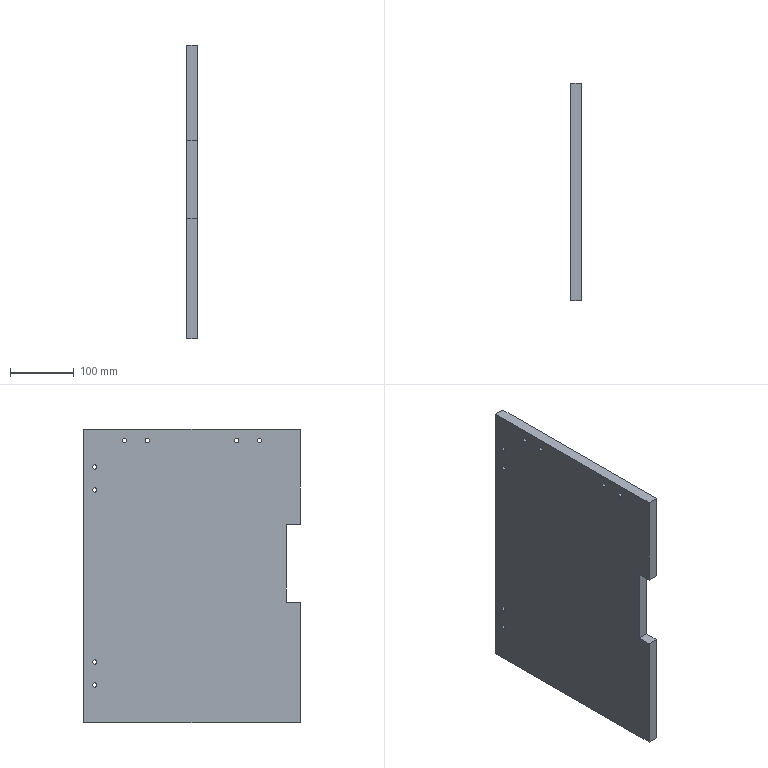Part | SolidWorks | features BaseBody 1 | 1 solid | 26 faces | box 16 x 340 x 460 mm | volume 2454807 mm3 | cylinder 16 | plane 10 | commonest cylinder face diameters 6.8 x16
STEP:
#1=CARTESIAN_POINT('',(0.,322.5,-167.6));
#2=VERTEX_POINT('',#1);
#3=CARTESIAN_POINT('',(0.,322.5,-174.4));
#4=VERTEX_POINT('',#3);
#5=CARTESIAN_POINT('',(0.,322.5,-171.));
#6=DIRECTION('',(1.,0.,0.));
#7=DIRECTION('',(0.,0.,-1.));
#8=AXIS2_PLACEMENT_3D('',#5,#6,#7);
#9=CIRCLE('',#8,3.4);
#10=EDGE_CURVE('',#2,#4,#9,.T.);
#11=ORIENTED_EDGE('',*,*,#10,.F.);
#12=CARTESIAN_POINT('',(16.,322.5,-167.6));
#13=VERTEX_POINT('',#12);
#14=CARTESIAN_POINT('',(16.,322.5,-167.6));
#15=DIRECTION('',(1.,0.,0.));
#16=VECTOR('',#15,1000.);
#17=LINE('',#14,#16);
#18=EDGE_CURVE('',#2,#13,#17,.T.);
#19=ORIENTED_EDGE('',*,*,#18,.T.);
#20=CARTESIAN_POINT('',(16.,322.5,-174.4));
#21=VERTEX_POINT('',#20);
#22=CARTESIAN_POINT('',(16.,322.5,-171.));
#23=DIRECTION('',(-1.,0.,0.));
#24=DIRECTION('',(0.,0.,-1.));
#25=AXIS2_PLACEMENT_3D('',#22,#23,#24);
#26=CIRCLE('',#25,3.4);
#27=EDGE_CURVE('',#21,#13,#26,.T.);
#28=ORIENTED_EDGE('',*,*,#27,.F.);
#29=CARTESIAN_POINT('',(16.,322.5,-174.4));
#30=DIRECTION('',(1.,0.,0.));
#31=VECTOR('',#30,1000.);
#32=LINE('',#29,#31);
#33=EDGE_CURVE('',#4,#21,#32,.T.);
#34=ORIENTED_EDGE('',*,*,#33,.F.);
#35=EDGE_LOOP('',(#11,#19,#28,#34));
#36=FACE_OUTER_BOUND('',#35,.T.);
#37=CARTESIAN_POINT('',(16.,322.5,-171.));
#38=DIRECTION('',(1.,0.,0.));
#39=DIRECTION('',(0.,0.,-1.));
#40=AXIS2_PLACEMENT_3D('',#37,#38,#39);
#41=CYLINDRICAL_SURFACE('',#40,3.4);
#42=ADVANCED_FACE('',(#36),#41,.F.);
#43=CARTESIAN_POINT('',(0.,322.5,-131.6));
#44=VERTEX_POINT('',#43);
#45=CARTESIAN_POINT('',(0.,322.5,-138.4));
#46=VERTEX_POINT('',#45);
#47=CARTESIAN_POINT('',(0.,322.5,-135.));
#48=DIRECTION('',(1.,0.,0.));
#49=DIRECTION('',(0.,0.,-1.));
#50=AXIS2_PLACEMENT_3D('',#47,#48,#49);
#51=CIRCLE('',#50,3.4);
#52=EDGE_CURVE('',#44,#46,#51,.T.);
#53=ORIENTED_EDGE('',*,*,#52,.F.);
#54=CARTESIAN_POINT('',(16.,322.5,-131.6));
#55=VERTEX_POINT('',#54);
#56=CARTESIAN_POINT('',(16.,322.5,-131.6));
#57=DIRECTION('',(1.,0.,0.));
#58=VECTOR('',#57,1000.);
#59=LINE('',#56,#58);
#60=EDGE_CURVE('',#44,#55,#59,.T.);
#61=ORIENTED_EDGE('',*,*,#60,.T.);
#62=CARTESIAN_POINT('',(16.,322.5,-138.4));
#63=VERTEX_POINT('',#62);
#64=CARTESIAN_POINT('',(16.,322.5,-135.));
#65=DIRECTION('',(-1.,0.,0.));
#66=DIRECTION('',(0.,0.,-1.));
#67=AXIS2_PLACEMENT_3D('',#64,#65,#66);
#68=CIRCLE('',#67,3.4);
#69=EDGE_CURVE('',#63,#55,#68,.T.);
#70=ORIENTED_EDGE('',*,*,#69,.F.);
#71=CARTESIAN_POINT('',(16.,322.5,-138.4));
#72=DIRECTION('',(1.,0.,0.));
#73=VECTOR('',#72,1000.);
#74=LINE('',#71,#73);
#75=EDGE_CURVE('',#46,#63,#74,.T.);
#76=ORIENTED_EDGE('',*,*,#75,.F.);
#77=EDGE_LOOP('',(#53,#61,#70,#76));
#78=FACE_OUTER_BOUND('',#77,.T.);
#79=CARTESIAN_POINT('',(16.,322.5,-135.));
#80=DIRECTION('',(1.,0.,0.));
#81=DIRECTION('',(0.,0.,-1.));
#82=AXIS2_PLACEMENT_3D('',#79,#80,#81);
#83=CYLINDRICAL_SURFACE('',#82,3.4);
#84=ADVANCED_FACE('',(#78),#83,.F.);
#85=CARTESIAN_POINT('',(0.,322.5,138.4));
#86=VERTEX_POINT('',#85);
#87=CARTESIAN_POINT('',(0.,322.5,131.6));
#88=VERTEX_POINT('',#87);
#89=CARTESIAN_POINT('',(0.,322.5,135.));
#90=DIRECTION('',(1.,0.,0.));
#91=DIRECTION('',(0.,0.,-1.));
#92=AXIS2_PLACEMENT_3D('',#89,#90,#91);
#93=CIRCLE('',#92,3.4);
#94=EDGE_CURVE('',#86,#88,#93,.T.);
#95=ORIENTED_EDGE('',*,*,#94,.F.);
#96=CARTESIAN_POINT('',(16.,322.5,138.4));
#97=VERTEX_POINT('',#96);
#98=CARTESIAN_POINT('',(16.,322.5,138.4));
#99=DIRECTION('',(1.,0.,0.));
#100=VECTOR('',#99,1000.);
#101=LINE('',#98,#100);
#102=EDGE_CURVE('',#86,#97,#101,.T.);
#103=ORIENTED_EDGE('',*,*,#102,.T.);
#104=CARTESIAN_POINT('',(16.,322.5,131.6));
#105=VERTEX_POINT('',#104);
#106=CARTESIAN_POINT('',(16.,322.5,135.));
#107=DIRECTION('',(-1.,0.,0.));
#108=DIRECTION('',(0.,0.,-1.));
#109=AXIS2_PLACEMENT_3D('',#106,#107,#108);
#110=CIRCLE('',#109,3.4);
#111=EDGE_CURVE('',#105,#97,#110,.T.);
#112=ORIENTED_EDGE('',*,*,#111,.F.);
#113=CARTESIAN_POINT('',(16.,322.5,131.6));
#114=DIRECTION('',(1.,0.,0.));
#115=VECTOR('',#114,1000.);
#116=LINE('',#113,#115);
#117=EDGE_CURVE('',#88,#105,#116,.T.);
#118=ORIENTED_EDGE('',*,*,#117,.F.);
#119=EDGE_LOOP('',(#95,#103,#112,#118));
#120=FACE_OUTER_BOUND('',#119,.T.);
#121=CARTESIAN_POINT('',(16.,322.5,135.));
#122=DIRECTION('',(1.,0.,0.));
#123=DIRECTION('',(0.,0.,-1.));
#124=AXIS2_PLACEMENT_3D('',#121,#122,#123);
#125=CYLINDRICAL_SURFACE('',#124,3.4);
#126=ADVANCED_FACE('',(#120),#125,.F.);
#127=CARTESIAN_POINT('',(0.,322.5,174.4));
#128=VERTEX_POINT('',#127);
#129=CARTESIAN_POINT('',(0.,322.5,167.6));
#130=VERTEX_POINT('',#129);
#131=CARTESIAN_POINT('',(0.,322.5,171.));
#132=DIRECTION('',(1.,0.,0.));
#133=DIRECTION('',(0.,0.,-1.));
#134=AXIS2_PLACEMENT_3D('',#131,#132,#133);
#135=CIRCLE('',#134,3.4);
#136=EDGE_CURVE('',#128,#130,#135,.T.);
#137=ORIENTED_EDGE('',*,*,#136,.F.);
#138=CARTESIAN_POINT('',(16.,322.5,174.4));
#139=VERTEX_POINT('',#138);
#140=CARTESIAN_POINT('',(16.,322.5,174.4));
#141=DIRECTION('',(1.,0.,0.));
#142=VECTOR('',#141,1000.);
#143=LINE('',#140,#142);
#144=EDGE_CURVE('',#128,#139,#143,.T.);
#145=ORIENTED_EDGE('',*,*,#144,.T.);
#146=CARTESIAN_POINT('',(16.,322.5,167.6));
#147=VERTEX_POINT('',#146);
#148=CARTESIAN_POINT('',(16.,322.5,171.));
#149=DIRECTION('',(-1.,0.,0.));
#150=DIRECTION('',(0.,0.,-1.));
#151=AXIS2_PLACEMENT_3D('',#148,#149,#150);
#152=CIRCLE('',#151,3.4);
#153=EDGE_CURVE('',#147,#139,#152,.T.);
#154=ORIENTED_EDGE('',*,*,#153,.F.);
#155=CARTESIAN_POINT('',(16.,322.5,167.6));
#156=DIRECTION('',(1.,0.,0.));
#157=VECTOR('',#156,1000.);
#158=LINE('',#155,#157);
#159=EDGE_CURVE('',#130,#147,#158,.T.);
#160=ORIENTED_EDGE('',*,*,#159,.F.);
#161=EDGE_LOOP('',(#137,#145,#154,#160));
#162=FACE_OUTER_BOUND('',#161,.T.);
#163=CARTESIAN_POINT('',(16.,322.5,171.));
#164=DIRECTION('',(1.,0.,0.));
#165=DIRECTION('',(0.,0.,-1.));
#166=AXIS2_PLACEMENT_3D('',#163,#164,#165);
#167=CYLINDRICAL_SURFACE('',#166,3.4);
#168=ADVANCED_FACE('',(#162),#167,.F.);
#169=CARTESIAN_POINT('',(0.,64.,215.9));
#170=VERTEX_POINT('',#169);
#171=CARTESIAN_POINT('',(0.,64.,209.1));
#172=VERTEX_POINT('',#171);
#173=CARTESIAN_POINT('',(0.,64.,212.5));
#174=DIRECTION('',(1.,0.,0.));
#175=DIRECTION('',(0.,0.,-1.));
#176=AXIS2_PLACEMENT_3D('',#173,#174,#175);
#177=CIRCLE('',#176,3.4);
#178=EDGE_CURVE('',#170,#172,#177,.T.);
#179=ORIENTED_EDGE('',*,*,#178,.F.);
#180=CARTESIAN_POINT('',(16.,64.,215.9));
#181=VERTEX_POINT('',#180);
#182=CARTESIAN_POINT('',(16.,64.,215.9));
#183=DIRECTION('',(1.,0.,0.));
#184=VECTOR('',#183,1000.);
#185=LINE('',#182,#184);
#186=EDGE_CURVE('',#170,#181,#185,.T.);
#187=ORIENTED_EDGE('',*,*,#186,.T.);
#188=CARTESIAN_POINT('',(16.,64.,209.1));
#189=VERTEX_POINT('',#188);
#190=CARTESIAN_POINT('',(16.,64.,212.5));
#191=DIRECTION('',(-1.,0.,0.));
#192=DIRECTION('',(0.,0.,-1.));
#193=AXIS2_PLACEMENT_3D('',#190,#191,#192);
#194=CIRCLE('',#193,3.4);
#195=EDGE_CURVE('',#189,#181,#194,.T.);
#196=ORIENTED_EDGE('',*,*,#195,.F.);
#197=CARTESIAN_POINT('',(16.,64.,209.1));
#198=DIRECTION('',(1.,0.,0.));
#199=VECTOR('',#198,1000.);
#200=LINE('',#197,#199);
#201=EDGE_CURVE('',#172,#189,#200,.T.);
#202=ORIENTED_EDGE('',*,*,#201,.F.);
#203=EDGE_LOOP('',(#179,#187,#196,#202));
#204=FACE_OUTER_BOUND('',#203,.T.);
#205=CARTESIAN_POINT('',(16.,64.,212.5));
#206=DIRECTION('',(1.,0.,0.));
#207=DIRECTION('',(0.,0.,-1.));
#208=AXIS2_PLACEMENT_3D('',#205,#206,#207);
#209=CYLINDRICAL_SURFACE('',#208,3.4);
#210=ADVANCED_FACE('',(#204),#209,.F.);
#211=CARTESIAN_POINT('',(0.,100.,215.9));
#212=VERTEX_POINT('',#211);
#213=CARTESIAN_POINT('',(0.,100.,209.1));
#214=VERTEX_POINT('',#213);
#215=CARTESIAN_POINT('',(0.,100.,212.5));
#216=DIRECTION('',(1.,0.,0.));
#217=DIRECTION('',(0.,0.,-1.));
#218=AXIS2_PLACEMENT_3D('',#215,#216,#217);
#219=CIRCLE('',#218,3.4);
#220=EDGE_CURVE('',#212,#214,#219,.T.);
#221=ORIENTED_EDGE('',*,*,#220,.F.);
#222=CARTESIAN_POINT('',(16.,100.,215.9));
#223=VERTEX_POINT('',#222);
#224=CARTESIAN_POINT('',(16.,100.,215.9));
#225=DIRECTION('',(1.,0.,0.));
#226=VECTOR('',#225,1000.);
#227=LINE('',#224,#226);
#228=EDGE_CURVE('',#212,#223,#227,.T.);
#229=ORIENTED_EDGE('',*,*,#228,.T.);
#230=CARTESIAN_POINT('',(16.,100.,209.1));
#231=VERTEX_POINT('',#230);
#232=CARTESIAN_POINT('',(16.,100.,212.5));
#233=DIRECTION('',(-1.,0.,0.));
#234=DIRECTION('',(0.,0.,-1.));
#235=AXIS2_PLACEMENT_3D('',#232,#233,#234);
#236=CIRCLE('',#235,3.4);
#237=EDGE_CURVE('',#231,#223,#236,.T.);
#238=ORIENTED_EDGE('',*,*,#237,.F.);
#239=CARTESIAN_POINT('',(16.,100.,209.1));
#240=DIRECTION('',(1.,0.,0.));
#241=VECTOR('',#240,1000.);
#242=LINE('',#239,#241);
#243=EDGE_CURVE('',#214,#231,#242,.T.);
#244=ORIENTED_EDGE('',*,*,#243,.F.);
#245=EDGE_LOOP('',(#221,#229,#238,#244));
#246=FACE_OUTER_BOUND('',#245,.T.);
#247=CARTESIAN_POINT('',(16.,100.,212.5));
#248=DIRECTION('',(1.,0.,0.));
#249=DIRECTION('',(0.,0.,-1.));
#250=AXIS2_PLACEMENT_3D('',#247,#248,#249);
#251=CYLINDRICAL_SURFACE('',#250,3.4);
#252=ADVANCED_FACE('',(#246),#251,.F.);
#253=CARTESIAN_POINT('',(0.,240.,215.9));
#254=VERTEX_POINT('',#253);
#255=CARTESIAN_POINT('',(0.,240.,209.1));
#256=VERTEX_POINT('',#255);
#257=CARTESIAN_POINT('',(0.,240.,212.5));
#258=DIRECTION('',(1.,0.,0.));
#259=DIRECTION('',(0.,0.,-1.));
#260=AXIS2_PLACEMENT_3D('',#257,#258,#259);
#261=CIRCLE('',#260,3.4);
#262=EDGE_CURVE('',#254,#256,#261,.T.);
#263=ORIENTED_EDGE('',*,*,#262,.F.);
#264=CARTESIAN_POINT('',(16.,240.,215.9));
#265=VERTEX_POINT('',#264);
#266=CARTESIAN_POINT('',(16.,240.,215.9));
#267=DIRECTION('',(1.,0.,0.));
#268=VECTOR('',#267,1000.);
#269=LINE('',#266,#268);
#270=EDGE_CURVE('',#254,#265,#269,.T.);
#271=ORIENTED_EDGE('',*,*,#270,.T.);
#272=CARTESIAN_POINT('',(16.,240.,209.1));
#273=VERTEX_POINT('',#272);
#274=CARTESIAN_POINT('',(16.,240.,212.5));
#275=DIRECTION('',(-1.,0.,0.));
#276=DIRECTION('',(0.,0.,-1.));
#277=AXIS2_PLACEMENT_3D('',#274,#275,#276);
#278=CIRCLE('',#277,3.4);
#279=EDGE_CURVE('',#273,#265,#278,.T.);
#280=ORIENTED_EDGE('',*,*,#279,.F.);
#281=CARTESIAN_POINT('',(16.,240.,209.1));
#282=DIRECTION('',(1.,0.,0.));
#283=VECTOR('',#282,1000.);
#284=LINE('',#281,#283);
#285=EDGE_CURVE('',#256,#273,#284,.T.);
#286=ORIENTED_EDGE('',*,*,#285,.F.);
#287=EDGE_LOOP('',(#263,#271,#280,#286));
#288=FACE_OUTER_BOUND('',#287,.T.);
#289=CARTESIAN_POINT('',(16.,240.,212.5));
#290=DIRECTION('',(1.,0.,0.));
#291=DIRECTION('',(0.,0.,-1.));
#292=AXIS2_PLACEMENT_3D('',#289,#290,#291);
#293=CYLINDRICAL_SURFACE('',#292,3.4);
#294=ADVANCED_FACE('',(#288),#293,.F.);
#295=CARTESIAN_POINT('',(0.,276.,215.9));
#296=VERTEX_POINT('',#295);
#297=CARTESIAN_POINT('',(0.,276.,209.1));
#298=VERTEX_POINT('',#297);
#299=CARTESIAN_POINT('',(0.,276.,212.5));
#300=DIRECTION('',(1.,0.,0.));
#301=DIRECTION('',(0.,0.,-1.));
#302=AXIS2_PLACEMENT_3D('',#299,#300,#301);
#303=CIRCLE('',#302,3.4);
#304=EDGE_CURVE('',#296,#298,#303,.T.);
#305=ORIENTED_EDGE('',*,*,#304,.F.);
#306=CARTESIAN_POINT('',(16.,276.,215.9));
#307=VERTEX_POINT('',#306);
#308=CARTESIAN_POINT('',(16.,276.,215.9));
#309=DIRECTION('',(1.,0.,0.));
#310=VECTOR('',#309,1000.);
#311=LINE('',#308,#310);
#312=EDGE_CURVE('',#296,#307,#311,.T.);
#313=ORIENTED_EDGE('',*,*,#312,.T.);
#314=CARTESIAN_POINT('',(16.,276.,209.1));
#315=VERTEX_POINT('',#314);
#316=CARTESIAN_POINT('',(16.,276.,212.5));
#317=DIRECTION('',(-1.,0.,0.));
#318=DIRECTION('',(0.,0.,-1.));
#319=AXIS2_PLACEMENT_3D('',#316,#317,#318);
#320=CIRCLE('',#319,3.4);
#321=EDGE_CURVE('',#315,#307,#320,.T.);
#322=ORIENTED_EDGE('',*,*,#321,.F.);
#323=CARTESIAN_POINT('',(16.,276.,209.1));
#324=DIRECTION('',(1.,0.,0.));
#325=VECTOR('',#324,1000.);
#326=LINE('',#323,#325);
#327=EDGE_CURVE('',#298,#315,#326,.T.);
#328=ORIENTED_EDGE('',*,*,#327,.F.);
#329=EDGE_LOOP('',(#305,#313,#322,#328));
#330=FACE_OUTER_BOUND('',#329,.T.);
#331=CARTESIAN_POINT('',(16.,276.,212.5));
#332=DIRECTION('',(1.,0.,0.));
#333=DIRECTION('',(0.,0.,-1.));
#334=AXIS2_PLACEMENT_3D('',#331,#332,#333);
#335=CYLINDRICAL_SURFACE('',#334,3.4);
#336=ADVANCED_FACE('',(#330),#335,.F.);
#337=CARTESIAN_POINT('',(0.,340.,-230.));
#338=VERTEX_POINT('',#337);
#339=CARTESIAN_POINT('',(0.,0.,-230.));
#340=VERTEX_POINT('',#339);
#341=CARTESIAN_POINT('',(0.,0.,-230.));
#342=DIRECTION('',(0.,-1.,0.));
#343=VECTOR('',#342,1000.);
#344=LINE('',#341,#343);
#345=EDGE_CURVE('',#338,#340,#344,.T.);
#346=ORIENTED_EDGE('',*,*,#345,.T.);
#347=CARTESIAN_POINT('',(0.,0.,-41.));
#348=VERTEX_POINT('',#347);
#349=CARTESIAN_POINT('',(0.,0.,0.));
#350=DIRECTION('',(0.,0.,1.));
#351=VECTOR('',#350,1000.);
#352=LINE('',#349,#351);
#353=EDGE_CURVE('',#340,#348,#352,.T.);
#354=ORIENTED_EDGE('',*,*,#353,.T.);
#355=CARTESIAN_POINT('',(0.,22.,-41.));
#356=VERTEX_POINT('',#355);
#357=CARTESIAN_POINT('',(0.,0.,-41.));
#358=DIRECTION('',(0.,1.,0.));
#359=VECTOR('',#358,1000.);
#360=LINE('',#357,#359);
#361=EDGE_CURVE('',#348,#356,#360,.T.);
#362=ORIENTED_EDGE('',*,*,#361,.T.);
#363=CARTESIAN_POINT('',(0.,22.,81.));
#364=VERTEX_POINT('',#363);
#365=CARTESIAN_POINT('',(0.,22.,0.));
#366=DIRECTION('',(0.,0.,1.));
#367=VECTOR('',#366,1000.);
#368=LINE('',#365,#367);
#369=EDGE_CURVE('',#356,#364,#368,.T.);
#370=ORIENTED_EDGE('',*,*,#369,.T.);
#371=CARTESIAN_POINT('',(0.,0.,81.));
#372=VERTEX_POINT('',#371);
#373=CARTESIAN_POINT('',(0.,0.,81.));
#374=DIRECTION('',(0.,-1.,0.));
#375=VECTOR('',#374,1000.);
#376=LINE('',#373,#375);
#377=EDGE_CURVE('',#364,#372,#376,.T.);
#378=ORIENTED_EDGE('',*,*,#377,.T.);
#379=CARTESIAN_POINT('',(0.,0.,230.));
#380=VERTEX_POINT('',#379);
#381=CARTESIAN_POINT('',(0.,0.,0.));
#382=DIRECTION('',(0.,0.,1.));
#383=VECTOR('',#382,1000.);
#384=LINE('',#381,#383);
#385=EDGE_CURVE('',#372,#380,#384,.T.);
#386=ORIENTED_EDGE('',*,*,#385,.T.);
#387=CARTESIAN_POINT('',(0.,340.,230.));
#388=VERTEX_POINT('',#387);
#389=CARTESIAN_POINT('',(0.,0.,230.));
#390=DIRECTION('',(0.,1.,0.));
#391=VECTOR('',#390,1000.);
#392=LINE('',#389,#391);
#393=EDGE_CURVE('',#380,#388,#392,.T.);
#394=ORIENTED_EDGE('',*,*,#393,.T.);
#395=CARTESIAN_POINT('',(0.,340.,0.));
#396=DIRECTION('',(0.,0.,-1.));
#397=VECTOR('',#396,1000.);
#398=LINE('',#395,#397);
#399=EDGE_CURVE('',#388,#338,#398,.T.);
#400=ORIENTED_EDGE('',*,*,#399,.T.);
#401=EDGE_LOOP('',(#346,#354,#362,#370,#378,#386,#394,#400));
#402=FACE_OUTER_BOUND('',#401,.T.);
#403=CARTESIAN_POINT('',(0.,322.5,-171.));
#404=DIRECTION('',(1.,0.,0.));
#405=DIRECTION('',(0.,0.,-1.));
#406=AXIS2_PLACEMENT_3D('',#403,#404,#405);
#407=CIRCLE('',#406,3.4);
#408=EDGE_CURVE('',#4,#2,#407,.T.);
#409=ORIENTED_EDGE('',*,*,#408,.T.);
#410=ORIENTED_EDGE('',*,*,#10,.T.);
#411=EDGE_LOOP('',(#409,#410));
#412=FACE_BOUND('',#411,.T.);
#413=CARTESIAN_POINT('',(0.,322.5,-135.));
#414=DIRECTION('',(1.,0.,0.));
#415=DIRECTION('',(0.,0.,-1.));
#416=AXIS2_PLACEMENT_3D('',#413,#414,#415);
#417=CIRCLE('',#416,3.4);
#418=EDGE_CURVE('',#46,#44,#417,.T.);
#419=ORIENTED_EDGE('',*,*,#418,.T.);
#420=ORIENTED_EDGE('',*,*,#52,.T.);
#421=EDGE_LOOP('',(#419,#420));
#422=FACE_BOUND('',#421,.T.);
#423=CARTESIAN_POINT('',(0.,322.5,135.));
#424=DIRECTION('',(1.,0.,0.));
#425=DIRECTION('',(0.,0.,-1.));
#426=AXIS2_PLACEMENT_3D('',#423,#424,#425);
#427=CIRCLE('',#426,3.4);
#428=EDGE_CURVE('',#88,#86,#427,.T.);
#429=ORIENTED_EDGE('',*,*,#428,.T.);
#430=ORIENTED_EDGE('',*,*,#94,.T.);
#431=EDGE_LOOP('',(#429,#430));
#432=FACE_BOUND('',#431,.T.);
#433=CARTESIAN_POINT('',(0.,322.5,171.));
#434=DIRECTION('',(1.,0.,0.));
#435=DIRECTION('',(0.,0.,-1.));
#436=AXIS2_PLACEMENT_3D('',#433,#434,#435);
#437=CIRCLE('',#436,3.4);
#438=EDGE_CURVE('',#130,#128,#437,.T.);
#439=ORIENTED_EDGE('',*,*,#438,.T.);
#440=ORIENTED_EDGE('',*,*,#136,.T.);
#441=EDGE_LOOP('',(#439,#440));
#442=FACE_BOUND('',#441,.T.);
#443=CARTESIAN_POINT('',(0.,64.,212.5));
#444=DIRECTION('',(1.,0.,0.));
#445=DIRECTION('',(0.,0.,-1.));
#446=AXIS2_PLACEMENT_3D('',#443,#444,#445);
#447=CIRCLE('',#446,3.4);
#448=EDGE_CURVE('',#172,#170,#447,.T.);
#449=ORIENTED_EDGE('',*,*,#448,.T.);
#450=ORIENTED_EDGE('',*,*,#178,.T.);
#451=EDGE_LOOP('',(#449,#450));
#452=FACE_BOUND('',#451,.T.);
#453=CARTESIAN_POINT('',(0.,100.,212.5));
#454=DIRECTION('',(1.,0.,0.));
#455=DIRECTION('',(0.,0.,-1.));
#456=AXIS2_PLACEMENT_3D('',#453,#454,#455);
#457=CIRCLE('',#456,3.4);
#458=EDGE_CURVE('',#214,#212,#457,.T.);
#459=ORIENTED_EDGE('',*,*,#458,.T.);
#460=ORIENTED_EDGE('',*,*,#220,.T.);
#461=EDGE_LOOP('',(#459,#460));
#462=FACE_BOUND('',#461,.T.);
#463=CARTESIAN_POINT('',(0.,240.,212.5));
#464=DIRECTION('',(1.,0.,0.));
#465=DIRECTION('',(0.,0.,-1.));
#466=AXIS2_PLACEMENT_3D('',#463,#464,#465);
#467=CIRCLE('',#466,3.4);
#468=EDGE_CURVE('',#256,#254,#467,.T.);
#469=ORIENTED_EDGE('',*,*,#468,.T.);
#470=ORIENTED_EDGE('',*,*,#262,.T.);
#471=EDGE_LOOP('',(#469,#470));
#472=FACE_BOUND('',#471,.T.);
#473=CARTESIAN_POINT('',(0.,276.,212.5));
#474=DIRECTION('',(1.,0.,0.));
#475=DIRECTION('',(0.,0.,-1.));
#476=AXIS2_PLACEMENT_3D('',#473,#474,#475);
#477=CIRCLE('',#476,3.4);
#478=EDGE_CURVE('',#298,#296,#477,.T.);
#479=ORIENTED_EDGE('',*,*,#478,.T.);
#480=ORIENTED_EDGE('',*,*,#304,.T.);
#481=EDGE_LOOP('',(#479,#480));
#482=FACE_BOUND('',#481,.T.);
#483=CARTESIAN_POINT('',(0.,0.,0.));
#484=DIRECTION('',(-1.,0.,0.));
#485=DIRECTION('',(0.,0.,1.));
#486=AXIS2_PLACEMENT_3D('',#483,#484,#485);
#487=PLANE('',#486);
#488=ADVANCED_FACE('',(#402,#412,#422,#432,#442,#452,#462,#472,#482),#487,.T.);
#489=CARTESIAN_POINT('',(16.,0.,-41.));
#490=VERTEX_POINT('',#489);
#491=CARTESIAN_POINT('',(16.,0.,-41.));
#492=DIRECTION('',(1.,0.,0.));
#493=VECTOR('',#492,1000.);
#494=LINE('',#491,#493);
#495=EDGE_CURVE('',#348,#490,#494,.T.);
#496=ORIENTED_EDGE('',*,*,#495,.F.);
#497=ORIENTED_EDGE('',*,*,#353,.F.);
#498=CARTESIAN_POINT('',(16.,0.,-230.));
#499=VERTEX_POINT('',#498);
#500=CARTESIAN_POINT('',(16.,0.,-230.));
#501=DIRECTION('',(-1.,0.,0.));
#502=VECTOR('',#501,1000.);
#503=LINE('',#500,#502);
#504=EDGE_CURVE('',#499,#340,#503,.T.);
#505=ORIENTED_EDGE('',*,*,#504,.F.);
#506=CARTESIAN_POINT('',(16.,0.,230.));
#507=DIRECTION('',(0.,0.,-1.));
#508=VECTOR('',#507,1000.);
#509=LINE('',#506,#508);
#510=EDGE_CURVE('',#490,#499,#509,.T.);
#511=ORIENTED_EDGE('',*,*,#510,.F.);
#512=EDGE_LOOP('',(#496,#497,#505,#511));
#513=FACE_OUTER_BOUND('',#512,.T.);
#514=CARTESIAN_POINT('',(16.,0.,230.));
#515=DIRECTION('',(0.,1.,0.));
#516=DIRECTION('',(0.,0.,1.));
#517=AXIS2_PLACEMENT_3D('',#514,#515,#516);
#518=PLANE('',#517);
#519=ADVANCED_FACE('',(#513),#518,.F.);
#520=CARTESIAN_POINT('',(16.,340.,-230.));
#521=VERTEX_POINT('',#520);
#522=CARTESIAN_POINT('',(16.,340.,-230.));
#523=DIRECTION('',(-1.,0.,0.));
#524=VECTOR('',#523,1000.);
#525=LINE('',#522,#524);
#526=EDGE_CURVE('',#521,#338,#525,.T.);
#527=ORIENTED_EDGE('',*,*,#526,.F.);
#528=CARTESIAN_POINT('',(16.,340.,-230.));
#529=DIRECTION('',(0.,1.,0.));
#530=VECTOR('',#529,1000.);
#531=LINE('',#528,#530);
#532=EDGE_CURVE('',#499,#521,#531,.T.);
#533=ORIENTED_EDGE('',*,*,#532,.F.);
#534=ORIENTED_EDGE('',*,*,#504,.T.);
#535=ORIENTED_EDGE('',*,*,#345,.F.);
#536=EDGE_LOOP('',(#527,#533,#534,#535));
#537=FACE_OUTER_BOUND('',#536,.T.);
#538=CARTESIAN_POINT('',(16.,340.,-230.));
#539=DIRECTION('',(0.,0.,1.));
#540=DIRECTION('',(0.,-1.,0.));
#541=AXIS2_PLACEMENT_3D('',#538,#539,#540);
#542=PLANE('',#541);
#543=ADVANCED_FACE('',(#537),#542,.F.);
#544=CARTESIAN_POINT('',(16.,340.,230.));
#545=VERTEX_POINT('',#544);
#546=CARTESIAN_POINT('',(16.,340.,230.));
#547=DIRECTION('',(-1.,0.,0.));
#548=VECTOR('',#547,1000.);
#549=LINE('',#546,#548);
#550=EDGE_CURVE('',#545,#388,#549,.T.);
#551=ORIENTED_EDGE('',*,*,#550,.F.);
#552=CARTESIAN_POINT('',(16.,340.,230.));
#553=DIRECTION('',(0.,0.,1.));
#554=VECTOR('',#553,1000.);
#555=LINE('',#552,#554);
#556=EDGE_CURVE('',#521,#545,#555,.T.);
#557=ORIENTED_EDGE('',*,*,#556,.F.);
#558=ORIENTED_EDGE('',*,*,#526,.T.);
#559=ORIENTED_EDGE('',*,*,#399,.F.);
#560=EDGE_LOOP('',(#551,#557,#558,#559));
#561=FACE_OUTER_BOUND('',#560,.T.);
#562=CARTESIAN_POINT('',(16.,340.,230.));
#563=DIRECTION('',(0.,-1.,0.));
#564=DIRECTION('',(0.,0.,-1.));
#565=AXIS2_PLACEMENT_3D('',#562,#563,#564);
#566=PLANE('',#565);
#567=ADVANCED_FACE('',(#561),#566,.F.);
#568=CARTESIAN_POINT('',(16.,0.,230.));
#569=VERTEX_POINT('',#568);
#570=CARTESIAN_POINT('',(16.,0.,230.));
#571=DIRECTION('',(-1.,0.,0.));
#572=VECTOR('',#571,1000.);
#573=LINE('',#570,#572);
#574=EDGE_CURVE('',#569,#380,#573,.T.);
#575=ORIENTED_EDGE('',*,*,#574,.F.);
#576=CARTESIAN_POINT('',(16.,0.,230.));
#577=DIRECTION('',(0.,-1.,0.));
#578=VECTOR('',#577,1000.);
#579=LINE('',#576,#578);
#580=EDGE_CURVE('',#545,#569,#579,.T.);
#581=ORIENTED_EDGE('',*,*,#580,.F.);
#582=ORIENTED_EDGE('',*,*,#550,.T.);
#583=ORIENTED_EDGE('',*,*,#393,.F.);
#584=EDGE_LOOP('',(#575,#581,#582,#583));
#585=FACE_OUTER_BOUND('',#584,.T.);
#586=CARTESIAN_POINT('',(16.,0.,230.));
#587=DIRECTION('',(0.,0.,-1.));
#588=DIRECTION('',(0.,1.,0.));
#589=AXIS2_PLACEMENT_3D('',#586,#587,#588);
#590=PLANE('',#589);
#591=ADVANCED_FACE('',(#585),#590,.F.);
#592=CARTESIAN_POINT('',(16.,0.,81.));
#593=VERTEX_POINT('',#592);
#594=CARTESIAN_POINT('',(16.,0.,81.));
#595=DIRECTION('',(-1.,0.,0.));
#596=VECTOR('',#595,1000.);
#597=LINE('',#594,#596);
#598=EDGE_CURVE('',#593,#372,#597,.T.);
#599=ORIENTED_EDGE('',*,*,#598,.F.);
#600=CARTESIAN_POINT('',(16.,0.,230.));
#601=DIRECTION('',(0.,0.,-1.));
#602=VECTOR('',#601,1000.);
#603=LINE('',#600,#602);
#604=EDGE_CURVE('',#569,#593,#603,.T.);
#605=ORIENTED_EDGE('',*,*,#604,.F.);
#606=ORIENTED_EDGE('',*,*,#574,.T.);
#607=ORIENTED_EDGE('',*,*,#385,.F.);
#608=EDGE_LOOP('',(#599,#605,#606,#607));
#609=FACE_OUTER_BOUND('',#608,.T.);
#610=CARTESIAN_POINT('',(16.,0.,230.));
#611=DIRECTION('',(0.,1.,0.));
#612=DIRECTION('',(0.,0.,1.));
#613=AXIS2_PLACEMENT_3D('',#610,#611,#612);
#614=PLANE('',#613);
#615=ADVANCED_FACE('',(#609),#614,.F.);
#616=ORIENTED_EDGE('',*,*,#598,.T.);
#617=ORIENTED_EDGE('',*,*,#377,.F.);
#618=CARTESIAN_POINT('',(16.,22.,81.));
#619=VERTEX_POINT('',#618);
#620=CARTESIAN_POINT('',(0.,22.,81.));
#621=DIRECTION('',(-1.,0.,0.));
#622=VECTOR('',#621,1000.);
#623=LINE('',#620,#622);
#624=EDGE_CURVE('',#619,#364,#623,.T.);
#625=ORIENTED_EDGE('',*,*,#624,.F.);
#626=CARTESIAN_POINT('',(16.,0.,81.));
#627=DIRECTION('',(0.,1.,0.));
#628=VECTOR('',#627,1000.);
#629=LINE('',#626,#628);
#630=EDGE_CURVE('',#593,#619,#629,.T.);
#631=ORIENTED_EDGE('',*,*,#630,.F.);
#632=EDGE_LOOP('',(#616,#617,#625,#631));
#633=FACE_OUTER_BOUND('',#632,.T.);
#634=CARTESIAN_POINT('',(0.,0.,81.));
#635=DIRECTION('',(0.,0.,1.));
#636=DIRECTION('',(1.,0.,0.));
#637=AXIS2_PLACEMENT_3D('',#634,#635,#636);
#638=PLANE('',#637);
#639=ADVANCED_FACE('',(#633),#638,.F.);
#640=ORIENTED_EDGE('',*,*,#624,.T.);
#641=ORIENTED_EDGE('',*,*,#369,.F.);
#642=CARTESIAN_POINT('',(16.,22.,-41.));
#643=VERTEX_POINT('',#642);
#644=CARTESIAN_POINT('',(0.,22.,-41.));
#645=DIRECTION('',(-1.,0.,0.));
#646=VECTOR('',#645,1000.);
#647=LINE('',#644,#646);
#648=EDGE_CURVE('',#643,#356,#647,.T.);
#649=ORIENTED_EDGE('',*,*,#648,.F.);
#650=CARTESIAN_POINT('',(16.,22.,-41.));
#651=DIRECTION('',(0.,0.,-1.));
#652=VECTOR('',#651,1000.);
#653=LINE('',#650,#652);
#654=EDGE_CURVE('',#619,#643,#653,.T.);
#655=ORIENTED_EDGE('',*,*,#654,.F.);
#656=EDGE_LOOP('',(#640,#641,#649,#655));
#657=FACE_OUTER_BOUND('',#656,.T.);
#658=CARTESIAN_POINT('',(0.,22.,-41.));
#659=DIRECTION('',(0.,1.,0.));
#660=DIRECTION('',(0.,0.,1.));
#661=AXIS2_PLACEMENT_3D('',#658,#659,#660);
#662=PLANE('',#661);
#663=ADVANCED_FACE('',(#657),#662,.F.);
#664=ORIENTED_EDGE('',*,*,#648,.T.);
#665=ORIENTED_EDGE('',*,*,#361,.F.);
#666=ORIENTED_EDGE('',*,*,#495,.T.);
#667=CARTESIAN_POINT('',(16.,0.,-41.));
#668=DIRECTION('',(0.,-1.,0.));
#669=VECTOR('',#668,1000.);
#670=LINE('',#667,#669);
#671=EDGE_CURVE('',#643,#490,#670,.T.);
#672=ORIENTED_EDGE('',*,*,#671,.F.);
#673=EDGE_LOOP('',(#664,#665,#666,#672));
#674=FACE_OUTER_BOUND('',#673,.T.);
#675=CARTESIAN_POINT('',(0.,0.,-41.));
#676=DIRECTION('',(0.,0.,-1.));
#677=DIRECTION('',(-1.,0.,0.));
#678=AXIS2_PLACEMENT_3D('',#675,#676,#677);
#679=PLANE('',#678);
#680=ADVANCED_FACE('',(#674),#679,.F.);
#681=ORIENTED_EDGE('',*,*,#18,.F.);
#682=ORIENTED_EDGE('',*,*,#408,.F.);
#683=ORIENTED_EDGE('',*,*,#33,.T.);
#684=CARTESIAN_POINT('',(16.,322.5,-171.));
#685=DIRECTION('',(-1.,0.,0.));
#686=DIRECTION('',(0.,0.,-1.));
#687=AXIS2_PLACEMENT_3D('',#684,#685,#686);
#688=CIRCLE('',#687,3.4);
#689=EDGE_CURVE('',#13,#21,#688,.T.);
#690=ORIENTED_EDGE('',*,*,#689,.F.);
#691=EDGE_LOOP('',(#681,#682,#683,#690));
#692=FACE_OUTER_BOUND('',#691,.T.);
#693=CARTESIAN_POINT('',(16.,322.5,-171.));
#694=DIRECTION('',(1.,0.,0.));
#695=DIRECTION('',(0.,0.,-1.));
#696=AXIS2_PLACEMENT_3D('',#693,#694,#695);
#697=CYLINDRICAL_SURFACE('',#696,3.4);
#698=ADVANCED_FACE('',(#692),#697,.F.);
#699=ORIENTED_EDGE('',*,*,#60,.F.);
#700=ORIENTED_EDGE('',*,*,#418,.F.);
#701=ORIENTED_EDGE('',*,*,#75,.T.);
#702=CARTESIAN_POINT('',(16.,322.5,-135.));
#703=DIRECTION('',(-1.,0.,0.));
#704=DIRECTION('',(0.,0.,-1.));
#705=AXIS2_PLACEMENT_3D('',#702,#703,#704);
#706=CIRCLE('',#705,3.4);
#707=EDGE_CURVE('',#55,#63,#706,.T.);
#708=ORIENTED_EDGE('',*,*,#707,.F.);
#709=EDGE_LOOP('',(#699,#700,#701,#708));
#710=FACE_OUTER_BOUND('',#709,.T.);
#711=CARTESIAN_POINT('',(16.,322.5,-135.));
#712=DIRECTION('',(1.,0.,0.));
#713=DIRECTION('',(0.,0.,-1.));
#714=AXIS2_PLACEMENT_3D('',#711,#712,#713);
#715=CYLINDRICAL_SURFACE('',#714,3.4);
#716=ADVANCED_FACE('',(#710),#715,.F.);
#717=ORIENTED_EDGE('',*,*,#102,.F.);
#718=ORIENTED_EDGE('',*,*,#428,.F.);
#719=ORIENTED_EDGE('',*,*,#117,.T.);
#720=CARTESIAN_POINT('',(16.,322.5,135.));
#721=DIRECTION('',(-1.,0.,0.));
#722=DIRECTION('',(0.,0.,-1.));
#723=AXIS2_PLACEMENT_3D('',#720,#721,#722);
#724=CIRCLE('',#723,3.4);
#725=EDGE_CURVE('',#97,#105,#724,.T.);
#726=ORIENTED_EDGE('',*,*,#725,.F.);
#727=EDGE_LOOP('',(#717,#718,#719,#726));
#728=FACE_OUTER_BOUND('',#727,.T.);
#729=CARTESIAN_POINT('',(16.,322.5,135.));
#730=DIRECTION('',(1.,0.,0.));
#731=DIRECTION('',(0.,0.,-1.));
#732=AXIS2_PLACEMENT_3D('',#729,#730,#731);
#733=CYLINDRICAL_SURFACE('',#732,3.4);
#734=ADVANCED_FACE('',(#728),#733,.F.);
#735=ORIENTED_EDGE('',*,*,#144,.F.);
#736=ORIENTED_EDGE('',*,*,#438,.F.);
#737=ORIENTED_EDGE('',*,*,#159,.T.);
#738=CARTESIAN_POINT('',(16.,322.5,171.));
#739=DIRECTION('',(-1.,0.,0.));
#740=DIRECTION('',(0.,0.,-1.));
#741=AXIS2_PLACEMENT_3D('',#738,#739,#740);
#742=CIRCLE('',#741,3.4);
#743=EDGE_CURVE('',#139,#147,#742,.T.);
#744=ORIENTED_EDGE('',*,*,#743,.F.);
#745=EDGE_LOOP('',(#735,#736,#737,#744));
#746=FACE_OUTER_BOUND('',#745,.T.);
#747=CARTESIAN_POINT('',(16.,322.5,171.));
#748=DIRECTION('',(1.,0.,0.));
#749=DIRECTION('',(0.,0.,-1.));
#750=AXIS2_PLACEMENT_3D('',#747,#748,#749);
#751=CYLINDRICAL_SURFACE('',#750,3.4);
#752=ADVANCED_FACE('',(#746),#751,.F.);
#753=ORIENTED_EDGE('',*,*,#186,.F.);
#754=ORIENTED_EDGE('',*,*,#448,.F.);
#755=ORIENTED_EDGE('',*,*,#201,.T.);
#756=CARTESIAN_POINT('',(16.,64.,212.5));
#757=DIRECTION('',(-1.,0.,0.));
#758=DIRECTION('',(0.,0.,-1.));
#759=AXIS2_PLACEMENT_3D('',#756,#757,#758);
#760=CIRCLE('',#759,3.4);
#761=EDGE_CURVE('',#181,#189,#760,.T.);
#762=ORIENTED_EDGE('',*,*,#761,.F.);
#763=EDGE_LOOP('',(#753,#754,#755,#762));
#764=FACE_OUTER_BOUND('',#763,.T.);
#765=CARTESIAN_POINT('',(16.,64.,212.5));
#766=DIRECTION('',(1.,0.,0.));
#767=DIRECTION('',(0.,0.,-1.));
#768=AXIS2_PLACEMENT_3D('',#765,#766,#767);
#769=CYLINDRICAL_SURFACE('',#768,3.4);
#770=ADVANCED_FACE('',(#764),#769,.F.);
#771=ORIENTED_EDGE('',*,*,#228,.F.);
#772=ORIENTED_EDGE('',*,*,#458,.F.);
#773=ORIENTED_EDGE('',*,*,#243,.T.);
#774=CARTESIAN_POINT('',(16.,100.,212.5));
#775=DIRECTION('',(-1.,0.,0.));
#776=DIRECTION('',(0.,0.,-1.));
#777=AXIS2_PLACEMENT_3D('',#774,#775,#776);
#778=CIRCLE('',#777,3.4);
#779=EDGE_CURVE('',#223,#231,#778,.T.);
#780=ORIENTED_EDGE('',*,*,#779,.F.);
#781=EDGE_LOOP('',(#771,#772,#773,#780));
#782=FACE_OUTER_BOUND('',#781,.T.);
#783=CARTESIAN_POINT('',(16.,100.,212.5));
#784=DIRECTION('',(1.,0.,0.));
#785=DIRECTION('',(0.,0.,-1.));
#786=AXIS2_PLACEMENT_3D('',#783,#784,#785);
#787=CYLINDRICAL_SURFACE('',#786,3.4);
#788=ADVANCED_FACE('',(#782),#787,.F.);
#789=ORIENTED_EDGE('',*,*,#270,.F.);
#790=ORIENTED_EDGE('',*,*,#468,.F.);
#791=ORIENTED_EDGE('',*,*,#285,.T.);
#792=CARTESIAN_POINT('',(16.,240.,212.5));
#793=DIRECTION('',(-1.,0.,0.));
#794=DIRECTION('',(0.,0.,-1.));
#795=AXIS2_PLACEMENT_3D('',#792,#793,#794);
#796=CIRCLE('',#795,3.4);
#797=EDGE_CURVE('',#265,#273,#796,.T.);
#798=ORIENTED_EDGE('',*,*,#797,.F.);
#799=EDGE_LOOP('',(#789,#790,#791,#798));
#800=FACE_OUTER_BOUND('',#799,.T.);
#801=CARTESIAN_POINT('',(16.,240.,212.5));
#802=DIRECTION('',(1.,0.,0.));
#803=DIRECTION('',(0.,0.,-1.));
#804=AXIS2_PLACEMENT_3D('',#801,#802,#803);
#805=CYLINDRICAL_SURFACE('',#804,3.4);
#806=ADVANCED_FACE('',(#800),#805,.F.);
#807=ORIENTED_EDGE('',*,*,#312,.F.);
#808=ORIENTED_EDGE('',*,*,#478,.F.);
#809=ORIENTED_EDGE('',*,*,#327,.T.);
#810=CARTESIAN_POINT('',(16.,276.,212.5));
#811=DIRECTION('',(-1.,0.,0.));
#812=DIRECTION('',(0.,0.,-1.));
#813=AXIS2_PLACEMENT_3D('',#810,#811,#812);
#814=CIRCLE('',#813,3.4);
#815=EDGE_CURVE('',#307,#315,#814,.T.);
#816=ORIENTED_EDGE('',*,*,#815,.F.);
#817=EDGE_LOOP('',(#807,#808,#809,#816));
#818=FACE_OUTER_BOUND('',#817,.T.);
#819=CARTESIAN_POINT('',(16.,276.,212.5));
#820=DIRECTION('',(1.,0.,0.));
#821=DIRECTION('',(0.,0.,-1.));
#822=AXIS2_PLACEMENT_3D('',#819,#820,#821);
#823=CYLINDRICAL_SURFACE('',#822,3.4);
#824=ADVANCED_FACE('',(#818),#823,.F.);
#825=ORIENTED_EDGE('',*,*,#671,.T.);
#826=ORIENTED_EDGE('',*,*,#510,.T.);
#827=ORIENTED_EDGE('',*,*,#532,.T.);
#828=ORIENTED_EDGE('',*,*,#556,.T.);
#829=ORIENTED_EDGE('',*,*,#580,.T.);
#830=ORIENTED_EDGE('',*,*,#604,.T.);
#831=ORIENTED_EDGE('',*,*,#630,.T.);
#832=ORIENTED_EDGE('',*,*,#654,.T.);
#833=EDGE_LOOP('',(#825,#826,#827,#828,#829,#830,#831,#832));
#834=FACE_OUTER_BOUND('',#833,.T.);
#835=ORIENTED_EDGE('',*,*,#27,.T.);
#836=ORIENTED_EDGE('',*,*,#689,.T.);
#837=EDGE_LOOP('',(#835,#836));
#838=FACE_BOUND('',#837,.T.);
#839=ORIENTED_EDGE('',*,*,#69,.T.);
#840=ORIENTED_EDGE('',*,*,#707,.T.);
#841=EDGE_LOOP('',(#839,#840));
#842=FACE_BOUND('',#841,.T.);
#843=ORIENTED_EDGE('',*,*,#111,.T.);
#844=ORIENTED_EDGE('',*,*,#725,.T.);
#845=EDGE_LOOP('',(#843,#844));
#846=FACE_BOUND('',#845,.T.);
#847=ORIENTED_EDGE('',*,*,#153,.T.);
#848=ORIENTED_EDGE('',*,*,#743,.T.);
#849=EDGE_LOOP('',(#847,#848));
#850=FACE_BOUND('',#849,.T.);
#851=ORIENTED_EDGE('',*,*,#195,.T.);
#852=ORIENTED_EDGE('',*,*,#761,.T.);
#853=EDGE_LOOP('',(#851,#852));
#854=FACE_BOUND('',#853,.T.);
#855=ORIENTED_EDGE('',*,*,#237,.T.);
#856=ORIENTED_EDGE('',*,*,#779,.T.);
#857=EDGE_LOOP('',(#855,#856));
#858=FACE_BOUND('',#857,.T.);
#859=ORIENTED_EDGE('',*,*,#279,.T.);
#860=ORIENTED_EDGE('',*,*,#797,.T.);
#861=EDGE_LOOP('',(#859,#860));
#862=FACE_BOUND('',#861,.T.);
#863=ORIENTED_EDGE('',*,*,#321,.T.);
#864=ORIENTED_EDGE('',*,*,#815,.T.);
#865=EDGE_LOOP('',(#863,#864));
#866=FACE_BOUND('',#865,.T.);
#867=CARTESIAN_POINT('',(16.,0.,0.));
#868=DIRECTION('',(-1.,0.,0.));
#869=DIRECTION('',(0.,0.,1.));
#870=AXIS2_PLACEMENT_3D('',#867,#868,#869);
#871=PLANE('',#870);
#872=ADVANCED_FACE('',(#834,#838,#842,#846,#850,#854,#858,#862,#866),#871,.F.);
#873=CLOSED_SHELL('',(#42,#84,#126,#168,#210,#252,#294,#336,#488,#519,#543,#567,#591,#615,#639,#663,#680,#698,#716,#734,#752,#770,#788,#806,#824,#872));
#874=MANIFOLD_SOLID_BREP('',#873);
#875=CARTESIAN_POINT('',(0.,0.,0.));
#876=DIRECTION('',(0.,0.,1.));
#877=DIRECTION('',(1.,0.,0.));
#878=AXIS2_PLACEMENT_3D('',#875,#876,#877);
#879=(LENGTH_UNIT()NAMED_UNIT(*)SI_UNIT(.MILLI.,.METRE.));
#880=UNCERTAINTY_MEASURE_WITH_UNIT(LENGTH_MEASURE(0.00001),#879,'','');
#881=(NAMED_UNIT(*)PLANE_ANGLE_UNIT()SI_UNIT($,.RADIAN.));
#882=(NAMED_UNIT(*)SI_UNIT($,.STERADIAN.)SOLID_ANGLE_UNIT());
#883=(GEOMETRIC_REPRESENTATION_CONTEXT(3)GLOBAL_UNCERTAINTY_ASSIGNED_CONTEXT((#880))GLOBAL_UNIT_ASSIGNED_CONTEXT((#879,#881,#882))REPRESENTATION_CONTEXT('',''));
#884=ADVANCED_BREP_SHAPE_REPRESENTATION('',(#874,#878),#883);